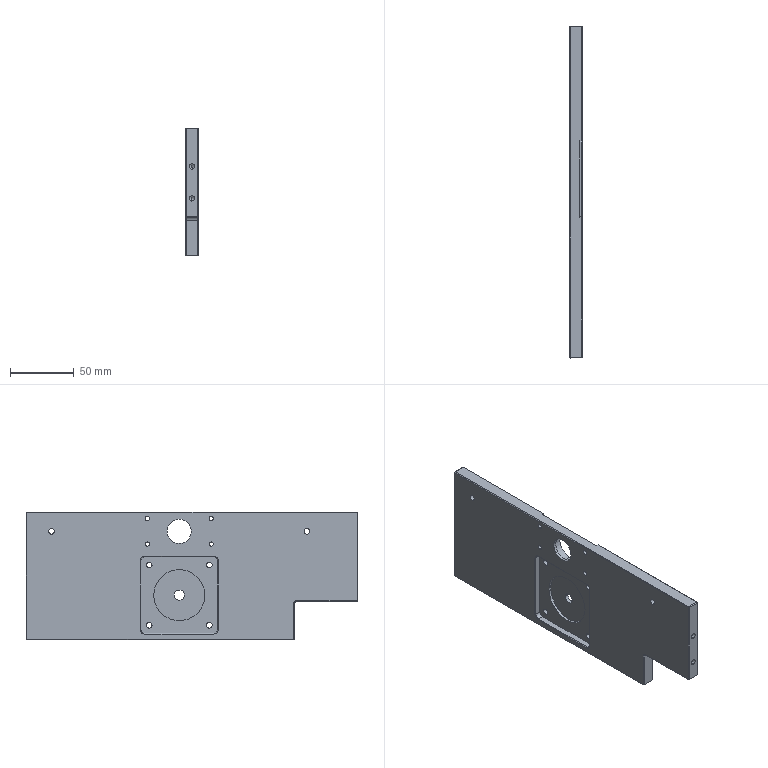Part | STEP file | 06-06 Driving feed support plate | 1 solid | 105 faces | box 10 x 260 x 100 mm | volume 216439 mm3 | plane 54 | cylinder 41 | cone 10 | commonest cylinder face diameters 4.5 x12 3.3 x8 2 x4 4.2 x4 6 x4 8 x2